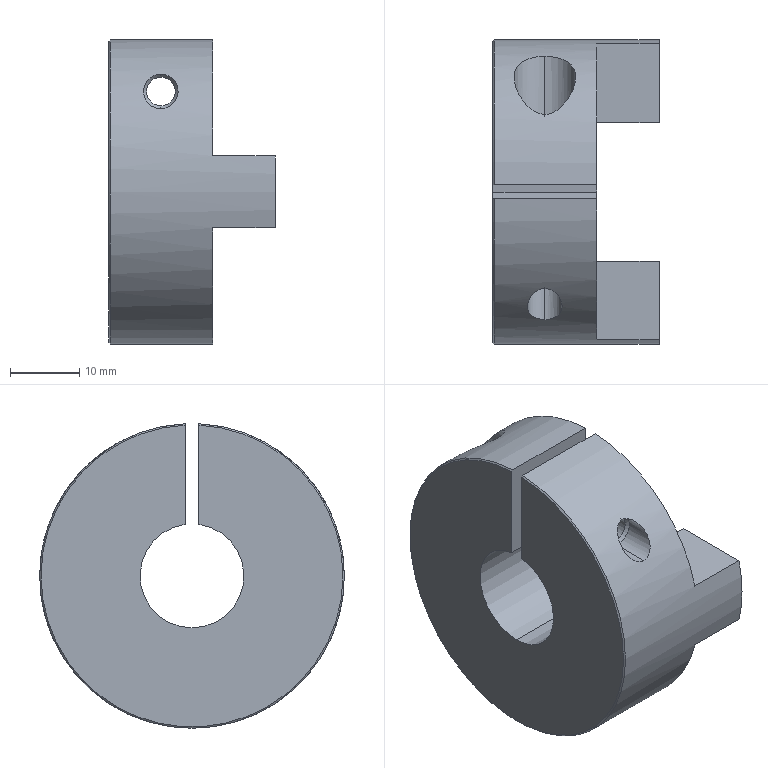Part | STEP file | 0244_Z_009_MFJC44-15-20_2 | 1 solid | 32 faces | box 24 x 44 x 43.977 mm | volume 20844 mm3 | cylinder 14 | plane 11 | cone 7 | commonest cylinder face diameters 5 x4 4.134 x2 8.9 x2 15 x2 22.5 x2 44 x2